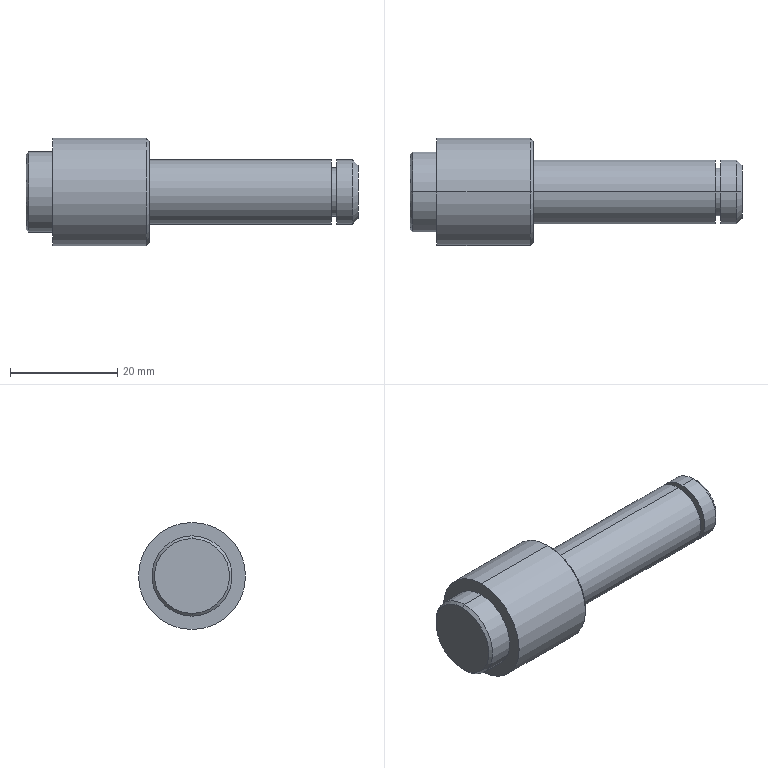Part | STEP file | 1 solid | 22 faces | box 62 x 20 x 20 mm | volume 10868 mm3 | cylinder 10 | cone 6 | plane 6 | commonest cylinder face diameters 12 x4 9 x2 15 x2 20 x2
STEP:
#1=CARTESIAN_POINT('',(0.,0.,0.));
#2=DIRECTION('',(0.,0.,1.));
#3=DIRECTION('',(1.,0.,0.));
#4=AXIS2_PLACEMENT_3D('',#1,#2,#3);
#5=CARTESIAN_POINT('',(23.,0.,-6.));
#6=VERTEX_POINT('',#5);
#7=CARTESIAN_POINT('',(23.,0.,6.));
#8=VERTEX_POINT('',#7);
#9=CARTESIAN_POINT('',(23.,0.,0.));
#10=DIRECTION('',(1.,0.,0.));
#11=DIRECTION('',(0.,0.,-1.));
#12=AXIS2_PLACEMENT_3D('',#9,#10,#11);
#13=CIRCLE('',#12,6.);
#14=CARTESIAN_POINT('',(40.,0.,0.));
#15=DIRECTION('',(1.,0.,0.));
#16=DIRECTION('',(0.,0.,-1.));
#17=AXIS2_PLACEMENT_3D('',#14,#15,#16);
#18=CYLINDRICAL_SURFACE('',#17,6.);
#19=CARTESIAN_POINT('',(0.,-17.));
#20=DIRECTION('',(1.,0.));
#21=VECTOR('',#20,1.);
#22=LINE('',#19,#21);
#23=(GEOMETRIC_REPRESENTATION_CONTEXT(2)PARAMETRIC_REPRESENTATION_CONTEXT()REPRESENTATION_CONTEXT('',''));
#24=DEFINITIONAL_REPRESENTATION('',(#22),#23);
#25=PCURVE('',#18,#24);
#26=CARTESIAN_POINT('',(23.,8.,0.));
#27=DIRECTION('',(1.,0.,0.));
#28=DIRECTION('',(0.,0.,-1.));
#29=AXIS2_PLACEMENT_3D('',#26,#27,#28);
#30=PLANE('',#29);
#31=CARTESIAN_POINT('',(0.,-8.));
#32=DIRECTION('',(1.,0.));
#33=AXIS2_PLACEMENT_2D('',#31,#32);
#34=CIRCLE('',#33,6.);
#35=(GEOMETRIC_REPRESENTATION_CONTEXT(2)PARAMETRIC_REPRESENTATION_CONTEXT()REPRESENTATION_CONTEXT('',''));
#36=DEFINITIONAL_REPRESENTATION('',(#34),#35);
#37=PCURVE('',#30,#36);
#38=SURFACE_CURVE('',#13,(#25,#37),.PCURVE_S1.);
#39=EDGE_CURVE('',#6,#8,#38,.T.);
#40=ORIENTED_EDGE('',*,*,#39,.T.);
#41=CARTESIAN_POINT('',(57.,0.,6.));
#42=VERTEX_POINT('',#41);
#43=CARTESIAN_POINT('',(40.,0.,6.));
#44=DIRECTION('',(1.,0.,0.));
#45=VECTOR('',#44,1.);
#46=LINE('',#43,#45);
#47=CARTESIAN_POINT('',(3.142,0.));
#48=DIRECTION('',(0.,1.));
#49=VECTOR('',#48,1.);
#50=LINE('',#47,#49);
#51=(GEOMETRIC_REPRESENTATION_CONTEXT(2)PARAMETRIC_REPRESENTATION_CONTEXT()REPRESENTATION_CONTEXT('',''));
#52=DEFINITIONAL_REPRESENTATION('',(#50),#51);
#53=PCURVE('',#18,#52);
#54=CARTESIAN_POINT('',(40.,0.,0.));
#55=DIRECTION('',(1.,0.,0.));
#56=DIRECTION('',(0.,0.,-1.));
#57=AXIS2_PLACEMENT_3D('',#54,#55,#56);
#58=CYLINDRICAL_SURFACE('',#57,6.);
#59=CARTESIAN_POINT('',(3.142,0.));
#60=DIRECTION('',(0.,1.));
#61=VECTOR('',#60,1.);
#62=LINE('',#59,#61);
#63=(GEOMETRIC_REPRESENTATION_CONTEXT(2)PARAMETRIC_REPRESENTATION_CONTEXT()REPRESENTATION_CONTEXT('',''));
#64=DEFINITIONAL_REPRESENTATION('',(#62),#63);
#65=PCURVE('',#58,#64);
#66=SURFACE_CURVE('',#46,(#53,#65),.PCURVE_S1.);
#67=EDGE_CURVE('',#8,#42,#66,.T.);
#68=ORIENTED_EDGE('',*,*,#67,.T.);
#69=CARTESIAN_POINT('',(57.,0.,-6.));
#70=VERTEX_POINT('',#69);
#71=CARTESIAN_POINT('',(57.,0.,0.));
#72=DIRECTION('',(-1.,0.,0.));
#73=DIRECTION('',(0.,0.,-1.));
#74=AXIS2_PLACEMENT_3D('',#71,#72,#73);
#75=CIRCLE('',#74,6.);
#76=CARTESIAN_POINT('',(6.283,17.));
#77=DIRECTION('',(-1.,0.));
#78=VECTOR('',#77,1.);
#79=LINE('',#76,#78);
#80=(GEOMETRIC_REPRESENTATION_CONTEXT(2)PARAMETRIC_REPRESENTATION_CONTEXT()REPRESENTATION_CONTEXT('',''));
#81=DEFINITIONAL_REPRESENTATION('',(#79),#80);
#82=PCURVE('',#18,#81);
#83=CARTESIAN_POINT('',(57.,5.25,0.));
#84=DIRECTION('',(1.,0.,0.));
#85=DIRECTION('',(0.,0.,-1.));
#86=AXIS2_PLACEMENT_3D('',#83,#84,#85);
#87=PLANE('',#86);
#88=CARTESIAN_POINT('',(6.,-5.25));
#89=CARTESIAN_POINT('',(6.,-15.642));
#90=CARTESIAN_POINT('',(-3.,-10.446));
#91=CARTESIAN_POINT('',(-12.,-5.25));
#92=CARTESIAN_POINT('',(-3.,-0.05385));
#93=CARTESIAN_POINT('',(6.,5.142));
#94=CARTESIAN_POINT('',(6.,-5.25));
#95=(BOUNDED_CURVE()B_SPLINE_CURVE(2,(#88,#89,#90,#91,#92,#93,#94),.UNSPECIFIED.,.T.,.F.)B_SPLINE_CURVE_WITH_KNOTS((1,2,2,2,2,1),(-2.094,0.,2.094,4.189,6.283,8.378),.UNSPECIFIED.)CURVE()GEOMETRIC_REPRESENTATION_ITEM()RATIONAL_B_SPLINE_CURVE((1.,0.5,1.,0.5,1.,0.5,1.))REPRESENTATION_ITEM(''));
#96=(GEOMETRIC_REPRESENTATION_CONTEXT(2)PARAMETRIC_REPRESENTATION_CONTEXT()REPRESENTATION_CONTEXT('',''));
#97=DEFINITIONAL_REPRESENTATION('',(#95),#96);
#98=PCURVE('',#87,#97);
#99=SURFACE_CURVE('',#75,(#82,#98),.PCURVE_S1.);
#100=EDGE_CURVE('',#42,#70,#99,.T.);
#101=ORIENTED_EDGE('',*,*,#100,.T.);
#102=CARTESIAN_POINT('',(40.,0.,-6.));
#103=DIRECTION('',(1.,0.,0.));
#104=VECTOR('',#103,1.);
#105=LINE('',#102,#104);
#106=CARTESIAN_POINT('',(0.,0.));
#107=DIRECTION('',(0.,1.));
#108=VECTOR('',#107,1.);
#109=LINE('',#106,#108);
#110=(GEOMETRIC_REPRESENTATION_CONTEXT(2)PARAMETRIC_REPRESENTATION_CONTEXT()REPRESENTATION_CONTEXT('',''));
#111=DEFINITIONAL_REPRESENTATION('',(#109),#110);
#112=PCURVE('',#18,#111);
#113=CARTESIAN_POINT('',(6.283,0.));
#114=DIRECTION('',(0.,1.));
#115=VECTOR('',#114,1.);
#116=LINE('',#113,#115);
#117=(GEOMETRIC_REPRESENTATION_CONTEXT(2)PARAMETRIC_REPRESENTATION_CONTEXT()REPRESENTATION_CONTEXT('',''));
#118=DEFINITIONAL_REPRESENTATION('',(#116),#117);
#119=PCURVE('',#58,#118);
#120=SURFACE_CURVE('',#105,(#112,#119),.PCURVE_S1.);
#121=EDGE_CURVE('',#6,#70,#120,.T.);
#122=ORIENTED_EDGE('',*,*,#121,.F.);
#123=EDGE_LOOP('',(#40,#68,#101,#122));
#124=FACE_BOUND('',#123,.T.);
#125=ADVANCED_FACE('',(#124),#18,.T.);
#126=CARTESIAN_POINT('',(23.,0.,-9.5));
#127=VERTEX_POINT('',#126);
#128=CARTESIAN_POINT('',(23.,0.,9.5));
#129=VERTEX_POINT('',#128);
#130=CARTESIAN_POINT('',(23.,0.,0.));
#131=DIRECTION('',(1.,0.,0.));
#132=DIRECTION('',(0.,0.,1.));
#133=AXIS2_PLACEMENT_3D('',#130,#131,#132);
#134=CIRCLE('',#133,9.5);
#135=CARTESIAN_POINT('',(22.5,0.,0.));
#136=DIRECTION('',(-1.,0.,0.));
#137=DIRECTION('',(0.,0.,1.));
#138=AXIS2_PLACEMENT_3D('',#135,#136,#137);
#139=CONICAL_SURFACE('',#138,10.,0.7854);
#140=CARTESIAN_POINT('',(6.283,-0.5));
#141=DIRECTION('',(-1.,0.));
#142=VECTOR('',#141,1.);
#143=LINE('',#140,#142);
#144=(GEOMETRIC_REPRESENTATION_CONTEXT(2)PARAMETRIC_REPRESENTATION_CONTEXT()REPRESENTATION_CONTEXT('',''));
#145=DEFINITIONAL_REPRESENTATION('',(#143),#144);
#146=PCURVE('',#139,#145);
#147=CARTESIAN_POINT('',(0.,-8.));
#148=DIRECTION('',(-1.,0.));
#149=AXIS2_PLACEMENT_2D('',#147,#148);
#150=CIRCLE('',#149,9.5);
#151=(GEOMETRIC_REPRESENTATION_CONTEXT(2)PARAMETRIC_REPRESENTATION_CONTEXT()REPRESENTATION_CONTEXT('',''));
#152=DEFINITIONAL_REPRESENTATION('',(#150),#151);
#153=PCURVE('',#30,#152);
#154=SURFACE_CURVE('',#134,(#146,#153),.PCURVE_S1.);
#155=EDGE_CURVE('',#127,#129,#154,.T.);
#156=ORIENTED_EDGE('',*,*,#155,.F.);
#157=CARTESIAN_POINT('',(22.5,0.,-10.));
#158=VERTEX_POINT('',#157);
#159=CARTESIAN_POINT('',(22.5,0.,-10.));
#160=DIRECTION('',(-0.7071,0.,-0.7071));
#161=VECTOR('',#160,1.);
#162=LINE('',#159,#161);
#163=CARTESIAN_POINT('',(3.142,0.));
#164=DIRECTION('',(0.,1.));
#165=VECTOR('',#164,1.);
#166=LINE('',#163,#165);
#167=(GEOMETRIC_REPRESENTATION_CONTEXT(2)PARAMETRIC_REPRESENTATION_CONTEXT()REPRESENTATION_CONTEXT('',''));
#168=DEFINITIONAL_REPRESENTATION('',(#166),#167);
#169=PCURVE('',#139,#168);
#170=CARTESIAN_POINT('',(22.5,0.,0.));
#171=DIRECTION('',(-1.,0.,0.));
#172=DIRECTION('',(0.,0.,1.));
#173=AXIS2_PLACEMENT_3D('',#170,#171,#172);
#174=CONICAL_SURFACE('',#173,10.,0.7854);
#175=CARTESIAN_POINT('',(3.142,0.));
#176=DIRECTION('',(0.,1.));
#177=VECTOR('',#176,1.);
#178=LINE('',#175,#177);
#179=(GEOMETRIC_REPRESENTATION_CONTEXT(2)PARAMETRIC_REPRESENTATION_CONTEXT()REPRESENTATION_CONTEXT('',''));
#180=DEFINITIONAL_REPRESENTATION('',(#178),#179);
#181=PCURVE('',#174,#180);
#182=SURFACE_CURVE('',#162,(#169,#181),.PCURVE_S1.);
#183=EDGE_CURVE('',#127,#158,#182,.T.);
#184=ORIENTED_EDGE('',*,*,#183,.T.);
#185=CARTESIAN_POINT('',(22.5,0.,10.));
#186=VERTEX_POINT('',#185);
#187=CARTESIAN_POINT('',(22.5,0.,0.));
#188=DIRECTION('',(1.,0.,0.));
#189=DIRECTION('',(0.,-1.,0.));
#190=AXIS2_PLACEMENT_3D('',#187,#188,#189);
#191=CIRCLE('',#190,10.);
#192=CARTESIAN_POINT('',(4.712,0.));
#193=DIRECTION('',(-1.,0.));
#194=VECTOR('',#193,1.);
#195=LINE('',#192,#194);
#196=(GEOMETRIC_REPRESENTATION_CONTEXT(2)PARAMETRIC_REPRESENTATION_CONTEXT()REPRESENTATION_CONTEXT('',''));
#197=DEFINITIONAL_REPRESENTATION('',(#195),#196);
#198=PCURVE('',#139,#197);
#199=CARTESIAN_POINT('',(14.,0.,0.));
#200=DIRECTION('',(1.,0.,0.));
#201=DIRECTION('',(0.,0.,-1.));
#202=AXIS2_PLACEMENT_3D('',#199,#200,#201);
#203=CYLINDRICAL_SURFACE('',#202,10.);
#204=CARTESIAN_POINT('',(-1.571,8.5));
#205=DIRECTION('',(1.,0.));
#206=VECTOR('',#205,1.);
#207=LINE('',#204,#206);
#208=(GEOMETRIC_REPRESENTATION_CONTEXT(2)PARAMETRIC_REPRESENTATION_CONTEXT()REPRESENTATION_CONTEXT('',''));
#209=DEFINITIONAL_REPRESENTATION('',(#207),#208);
#210=PCURVE('',#203,#209);
#211=SURFACE_CURVE('',#191,(#198,#210),.PCURVE_S1.);
#212=EDGE_CURVE('',#158,#186,#211,.T.);
#213=ORIENTED_EDGE('',*,*,#212,.T.);
#214=CARTESIAN_POINT('',(22.5,0.,10.));
#215=DIRECTION('',(-0.7071,0.,0.7071));
#216=VECTOR('',#215,1.);
#217=LINE('',#214,#216);
#218=CARTESIAN_POINT('',(0.,0.));
#219=DIRECTION('',(0.,1.));
#220=VECTOR('',#219,1.);
#221=LINE('',#218,#220);
#222=(GEOMETRIC_REPRESENTATION_CONTEXT(2)PARAMETRIC_REPRESENTATION_CONTEXT()REPRESENTATION_CONTEXT('',''));
#223=DEFINITIONAL_REPRESENTATION('',(#221),#222);
#224=PCURVE('',#139,#223);
#225=CARTESIAN_POINT('',(6.283,0.));
#226=DIRECTION('',(0.,1.));
#227=VECTOR('',#226,1.);
#228=LINE('',#225,#227);
#229=(GEOMETRIC_REPRESENTATION_CONTEXT(2)PARAMETRIC_REPRESENTATION_CONTEXT()REPRESENTATION_CONTEXT('',''));
#230=DEFINITIONAL_REPRESENTATION('',(#228),#229);
#231=PCURVE('',#174,#230);
#232=SURFACE_CURVE('',#217,(#224,#231),.PCURVE_S1.);
#233=EDGE_CURVE('',#129,#186,#232,.T.);
#234=ORIENTED_EDGE('',*,*,#233,.F.);
#235=EDGE_LOOP('',(#156,#184,#213,#234));
#236=FACE_BOUND('',#235,.T.);
#237=ADVANCED_FACE('',(#236),#139,.T.);
#238=CARTESIAN_POINT('',(57.,0.,4.5));
#239=VERTEX_POINT('',#238);
#240=CARTESIAN_POINT('',(57.,0.,-4.5));
#241=VERTEX_POINT('',#240);
#242=CARTESIAN_POINT('',(57.,0.,0.));
#243=DIRECTION('',(-1.,0.,0.));
#244=DIRECTION('',(0.,0.,-1.));
#245=AXIS2_PLACEMENT_3D('',#242,#243,#244);
#246=CIRCLE('',#245,4.5);
#247=CARTESIAN_POINT('',(57.5,0.,0.));
#248=DIRECTION('',(1.,0.,0.));
#249=DIRECTION('',(0.,0.,-1.));
#250=AXIS2_PLACEMENT_3D('',#247,#248,#249);
#251=CYLINDRICAL_SURFACE('',#250,4.5);
#252=CARTESIAN_POINT('',(6.283,-0.5));
#253=DIRECTION('',(-1.,0.));
#254=VECTOR('',#253,1.);
#255=LINE('',#252,#254);
#256=(GEOMETRIC_REPRESENTATION_CONTEXT(2)PARAMETRIC_REPRESENTATION_CONTEXT()REPRESENTATION_CONTEXT('',''));
#257=DEFINITIONAL_REPRESENTATION('',(#255),#256);
#258=PCURVE('',#251,#257);
#259=CARTESIAN_POINT('',(4.5,-5.25));
#260=CARTESIAN_POINT('',(4.5,-13.044));
#261=CARTESIAN_POINT('',(-2.25,-9.147));
#262=CARTESIAN_POINT('',(-9.,-5.25));
#263=CARTESIAN_POINT('',(-2.25,-1.353));
#264=CARTESIAN_POINT('',(4.5,2.544));
#265=CARTESIAN_POINT('',(4.5,-5.25));
#266=(BOUNDED_CURVE()B_SPLINE_CURVE(2,(#259,#260,#261,#262,#263,#264,#265),.UNSPECIFIED.,.T.,.F.)B_SPLINE_CURVE_WITH_KNOTS((1,2,2,2,2,1),(-2.094,0.,2.094,4.189,6.283,8.378),.UNSPECIFIED.)CURVE()GEOMETRIC_REPRESENTATION_ITEM()RATIONAL_B_SPLINE_CURVE((1.,0.5,1.,0.5,1.,0.5,1.))REPRESENTATION_ITEM(''));
#267=(GEOMETRIC_REPRESENTATION_CONTEXT(2)PARAMETRIC_REPRESENTATION_CONTEXT()REPRESENTATION_CONTEXT('',''));
#268=DEFINITIONAL_REPRESENTATION('',(#266),#267);
#269=PCURVE('',#87,#268);
#270=SURFACE_CURVE('',#246,(#258,#269),.PCURVE_S1.);
#271=EDGE_CURVE('',#239,#241,#270,.T.);
#272=ORIENTED_EDGE('',*,*,#271,.F.);
#273=CARTESIAN_POINT('',(58.,0.,4.5));
#274=VERTEX_POINT('',#273);
#275=CARTESIAN_POINT('',(57.5,0.,4.5));
#276=DIRECTION('',(1.,0.,0.));
#277=VECTOR('',#276,1.);
#278=LINE('',#275,#277);
#279=CARTESIAN_POINT('',(3.142,0.));
#280=DIRECTION('',(0.,1.));
#281=VECTOR('',#280,1.);
#282=LINE('',#279,#281);
#283=(GEOMETRIC_REPRESENTATION_CONTEXT(2)PARAMETRIC_REPRESENTATION_CONTEXT()REPRESENTATION_CONTEXT('',''));
#284=DEFINITIONAL_REPRESENTATION('',(#282),#283);
#285=PCURVE('',#251,#284);
#286=CARTESIAN_POINT('',(57.5,0.,0.));
#287=DIRECTION('',(1.,0.,0.));
#288=DIRECTION('',(0.,0.,-1.));
#289=AXIS2_PLACEMENT_3D('',#286,#287,#288);
#290=CYLINDRICAL_SURFACE('',#289,4.5);
#291=CARTESIAN_POINT('',(3.142,0.));
#292=DIRECTION('',(0.,1.));
#293=VECTOR('',#292,1.);
#294=LINE('',#291,#293);
#295=(GEOMETRIC_REPRESENTATION_CONTEXT(2)PARAMETRIC_REPRESENTATION_CONTEXT()REPRESENTATION_CONTEXT('',''));
#296=DEFINITIONAL_REPRESENTATION('',(#294),#295);
#297=PCURVE('',#290,#296);
#298=SURFACE_CURVE('',#278,(#285,#297),.PCURVE_S1.);
#299=EDGE_CURVE('',#239,#274,#298,.T.);
#300=ORIENTED_EDGE('',*,*,#299,.T.);
#301=CARTESIAN_POINT('',(58.,0.,-4.5));
#302=VERTEX_POINT('',#301);
#303=CARTESIAN_POINT('',(58.,0.,0.));
#304=DIRECTION('',(-1.,0.,0.));
#305=DIRECTION('',(0.,0.,-1.));
#306=AXIS2_PLACEMENT_3D('',#303,#304,#305);
#307=CIRCLE('',#306,4.5);
#308=CARTESIAN_POINT('',(6.283,0.5));
#309=DIRECTION('',(-1.,0.));
#310=VECTOR('',#309,1.);
#311=LINE('',#308,#310);
#312=(GEOMETRIC_REPRESENTATION_CONTEXT(2)PARAMETRIC_REPRESENTATION_CONTEXT()REPRESENTATION_CONTEXT('',''));
#313=DEFINITIONAL_REPRESENTATION('',(#311),#312);
#314=PCURVE('',#251,#313);
#315=CARTESIAN_POINT('',(58.,5.25,0.));
#316=DIRECTION('',(-1.,0.,0.));
#317=DIRECTION('',(0.,0.,1.));
#318=AXIS2_PLACEMENT_3D('',#315,#316,#317);
#319=PLANE('',#318);
#320=CARTESIAN_POINT('',(0.,-5.25));
#321=DIRECTION('',(-1.,0.));
#322=AXIS2_PLACEMENT_2D('',#320,#321);
#323=CIRCLE('',#322,4.5);
#324=(GEOMETRIC_REPRESENTATION_CONTEXT(2)PARAMETRIC_REPRESENTATION_CONTEXT()REPRESENTATION_CONTEXT('',''));
#325=DEFINITIONAL_REPRESENTATION('',(#323),#324);
#326=PCURVE('',#319,#325);
#327=SURFACE_CURVE('',#307,(#314,#326),.PCURVE_S1.);
#328=EDGE_CURVE('',#274,#302,#327,.T.);
#329=ORIENTED_EDGE('',*,*,#328,.T.);
#330=CARTESIAN_POINT('',(57.5,0.,-4.5));
#331=DIRECTION('',(1.,0.,0.));
#332=VECTOR('',#331,1.);
#333=LINE('',#330,#332);
#334=CARTESIAN_POINT('',(0.,0.));
#335=DIRECTION('',(0.,1.));
#336=VECTOR('',#335,1.);
#337=LINE('',#334,#336);
#338=(GEOMETRIC_REPRESENTATION_CONTEXT(2)PARAMETRIC_REPRESENTATION_CONTEXT()REPRESENTATION_CONTEXT('',''));
#339=DEFINITIONAL_REPRESENTATION('',(#337),#338);
#340=PCURVE('',#251,#339);
#341=CARTESIAN_POINT('',(6.283,0.));
#342=DIRECTION('',(0.,1.));
#343=VECTOR('',#342,1.);
#344=LINE('',#341,#343);
#345=(GEOMETRIC_REPRESENTATION_CONTEXT(2)PARAMETRIC_REPRESENTATION_CONTEXT()REPRESENTATION_CONTEXT('',''));
#346=DEFINITIONAL_REPRESENTATION('',(#344),#345);
#347=PCURVE('',#290,#346);
#348=SURFACE_CURVE('',#333,(#340,#347),.PCURVE_S1.);
#349=EDGE_CURVE('',#241,#302,#348,.T.);
#350=ORIENTED_EDGE('',*,*,#349,.F.);
#351=EDGE_LOOP('',(#272,#300,#329,#350));
#352=FACE_BOUND('',#351,.T.);
#353=ADVANCED_FACE('',(#352),#251,.T.);
#354=CARTESIAN_POINT('',(5.,0.,-10.));
#355=VERTEX_POINT('',#354);
#356=CARTESIAN_POINT('',(5.,0.,10.));
#357=VERTEX_POINT('',#356);
#358=CARTESIAN_POINT('',(5.,0.,0.));
#359=DIRECTION('',(1.,0.,0.));
#360=DIRECTION('',(0.,0.,-1.));
#361=AXIS2_PLACEMENT_3D('',#358,#359,#360);
#362=CIRCLE('',#361,10.);
#363=CARTESIAN_POINT('',(0.,-9.));
#364=DIRECTION('',(1.,0.));
#365=VECTOR('',#364,1.);
#366=LINE('',#363,#365);
#367=(GEOMETRIC_REPRESENTATION_CONTEXT(2)PARAMETRIC_REPRESENTATION_CONTEXT()REPRESENTATION_CONTEXT('',''));
#368=DEFINITIONAL_REPRESENTATION('',(#366),#367);
#369=PCURVE('',#203,#368);
#370=CARTESIAN_POINT('',(5.,8.75,0.));
#371=DIRECTION('',(-1.,0.,0.));
#372=DIRECTION('',(0.,0.,1.));
#373=AXIS2_PLACEMENT_3D('',#370,#371,#372);
#374=PLANE('',#373);
#375=CARTESIAN_POINT('',(-10.,-8.75));
#376=CARTESIAN_POINT('',(-10.,8.571));
#377=CARTESIAN_POINT('',(5.,-0.08975));
#378=CARTESIAN_POINT('',(20.,-8.75));
#379=CARTESIAN_POINT('',(5.,-17.41));
#380=CARTESIAN_POINT('',(-10.,-26.071));
#381=CARTESIAN_POINT('',(-10.,-8.75));
#382=(BOUNDED_CURVE()B_SPLINE_CURVE(2,(#375,#376,#377,#378,#379,#380,#381),.UNSPECIFIED.,.T.,.F.)B_SPLINE_CURVE_WITH_KNOTS((1,2,2,2,2,1),(-2.094,0.,2.094,4.189,6.283,8.378),.UNSPECIFIED.)CURVE()GEOMETRIC_REPRESENTATION_ITEM()RATIONAL_B_SPLINE_CURVE((1.,0.5,1.,0.5,1.,0.5,1.))REPRESENTATION_ITEM(''));
#383=(GEOMETRIC_REPRESENTATION_CONTEXT(2)PARAMETRIC_REPRESENTATION_CONTEXT()REPRESENTATION_CONTEXT('',''));
#384=DEFINITIONAL_REPRESENTATION('',(#382),#383);
#385=PCURVE('',#374,#384);
#386=SURFACE_CURVE('',#362,(#369,#385),.PCURVE_S1.);
#387=EDGE_CURVE('',#355,#357,#386,.T.);
#388=ORIENTED_EDGE('',*,*,#387,.T.);
#389=CARTESIAN_POINT('',(14.,0.,10.));
#390=DIRECTION('',(1.,0.,0.));
#391=VECTOR('',#390,1.);
#392=LINE('',#389,#391);
#393=CARTESIAN_POINT('',(3.142,0.));
#394=DIRECTION('',(0.,1.));
#395=VECTOR('',#394,1.);
#396=LINE('',#393,#395);
#397=(GEOMETRIC_REPRESENTATION_CONTEXT(2)PARAMETRIC_REPRESENTATION_CONTEXT()REPRESENTATION_CONTEXT('',''));
#398=DEFINITIONAL_REPRESENTATION('',(#396),#397);
#399=PCURVE('',#203,#398);
#400=CARTESIAN_POINT('',(14.,0.,0.));
#401=DIRECTION('',(1.,0.,0.));
#402=DIRECTION('',(0.,0.,-1.));
#403=AXIS2_PLACEMENT_3D('',#400,#401,#402);
#404=CYLINDRICAL_SURFACE('',#403,10.);
#405=CARTESIAN_POINT('',(3.142,0.));
#406=DIRECTION('',(0.,1.));
#407=VECTOR('',#406,1.);
#408=LINE('',#405,#407);
#409=(GEOMETRIC_REPRESENTATION_CONTEXT(2)PARAMETRIC_REPRESENTATION_CONTEXT()REPRESENTATION_CONTEXT('',''));
#410=DEFINITIONAL_REPRESENTATION('',(#408),#409);
#411=PCURVE('',#404,#410);
#412=SURFACE_CURVE('',#392,(#399,#411),.PCURVE_S1.);
#413=EDGE_CURVE('',#357,#186,#412,.T.);
#414=ORIENTED_EDGE('',*,*,#413,.T.);
#415=ORIENTED_EDGE('',*,*,#212,.F.);
#416=CARTESIAN_POINT('',(14.,0.,-10.));
#417=DIRECTION('',(1.,0.,0.));
#418=VECTOR('',#417,1.);
#419=LINE('',#416,#418);
#420=CARTESIAN_POINT('',(0.,0.));
#421=DIRECTION('',(0.,1.));
#422=VECTOR('',#421,1.);
#423=LINE('',#420,#422);
#424=(GEOMETRIC_REPRESENTATION_CONTEXT(2)PARAMETRIC_REPRESENTATION_CONTEXT()REPRESENTATION_CONTEXT('',''));
#425=DEFINITIONAL_REPRESENTATION('',(#423),#424);
#426=PCURVE('',#203,#425);
#427=CARTESIAN_POINT('',(6.283,0.));
#428=DIRECTION('',(0.,1.));
#429=VECTOR('',#428,1.);
#430=LINE('',#427,#429);
#431=(GEOMETRIC_REPRESENTATION_CONTEXT(2)PARAMETRIC_REPRESENTATION_CONTEXT()REPRESENTATION_CONTEXT('',''));
#432=DEFINITIONAL_REPRESENTATION('',(#430),#431);
#433=PCURVE('',#404,#432);
#434=SURFACE_CURVE('',#419,(#426,#433),.PCURVE_S1.);
#435=EDGE_CURVE('',#355,#158,#434,.T.);
#436=ORIENTED_EDGE('',*,*,#435,.F.);
#437=EDGE_LOOP('',(#388,#414,#415,#436));
#438=FACE_BOUND('',#437,.T.);
#439=ADVANCED_FACE('',(#438),#203,.T.);
#440=CARTESIAN_POINT('',(58.,0.,6.));
#441=VERTEX_POINT('',#440);
#442=CARTESIAN_POINT('',(58.,0.,-6.));
#443=VERTEX_POINT('',#442);
#444=CARTESIAN_POINT('',(58.,0.,0.));
#445=DIRECTION('',(-1.,0.,0.));
#446=DIRECTION('',(0.,0.,-1.));
#447=AXIS2_PLACEMENT_3D('',#444,#445,#446);
#448=CIRCLE('',#447,6.);
#449=CARTESIAN_POINT('',(59.5,0.,0.));
#450=DIRECTION('',(1.,0.,0.));
#451=DIRECTION('',(0.,0.,-1.));
#452=AXIS2_PLACEMENT_3D('',#449,#450,#451);
#453=CYLINDRICAL_SURFACE('',#452,6.);
#454=CARTESIAN_POINT('',(6.283,-1.5));
#455=DIRECTION('',(-1.,0.));
#456=VECTOR('',#455,1.);
#457=LINE('',#454,#456);
#458=(GEOMETRIC_REPRESENTATION_CONTEXT(2)PARAMETRIC_REPRESENTATION_CONTEXT()REPRESENTATION_CONTEXT('',''));
#459=DEFINITIONAL_REPRESENTATION('',(#457),#458);
#460=PCURVE('',#453,#459);
#461=CARTESIAN_POINT('',(0.,-5.25));
#462=DIRECTION('',(-1.,0.));
#463=AXIS2_PLACEMENT_2D('',#461,#462);
#464=CIRCLE('',#463,6.);
#465=(GEOMETRIC_REPRESENTATION_CONTEXT(2)PARAMETRIC_REPRESENTATION_CONTEXT()REPRESENTATION_CONTEXT('',''));
#466=DEFINITIONAL_REPRESENTATION('',(#464),#465);
#467=PCURVE('',#319,#466);
#468=SURFACE_CURVE('',#448,(#460,#467),.PCURVE_S1.);
#469=EDGE_CURVE('',#441,#443,#468,.T.);
#470=ORIENTED_EDGE('',*,*,#469,.F.);
#471=CARTESIAN_POINT('',(61.,0.,6.));
#472=VERTEX_POINT('',#471);
#473=CARTESIAN_POINT('',(59.5,0.,6.));
#474=DIRECTION('',(1.,0.,0.));
#475=VECTOR('',#474,1.);
#476=LINE('',#473,#475);
#477=CARTESIAN_POINT('',(3.142,0.));
#478=DIRECTION('',(0.,1.));
#479=VECTOR('',#478,1.);
#480=LINE('',#477,#479);
#481=(GEOMETRIC_REPRESENTATION_CONTEXT(2)PARAMETRIC_REPRESENTATION_CONTEXT()REPRESENTATION_CONTEXT('',''));
#482=DEFINITIONAL_REPRESENTATION('',(#480),#481);
#483=PCURVE('',#453,#482);
#484=CARTESIAN_POINT('',(59.5,0.,0.));
#485=DIRECTION('',(1.,0.,0.));
#486=DIRECTION('',(0.,0.,-1.));
#487=AXIS2_PLACEMENT_3D('',#484,#485,#486);
#488=CYLINDRICAL_SURFACE('',#487,6.);
#489=CARTESIAN_POINT('',(3.142,0.));
#490=DIRECTION('',(0.,1.));
#491=VECTOR('',#490,1.);
#492=LINE('',#489,#491);
#493=(GEOMETRIC_REPRESENTATION_CONTEXT(2)PARAMETRIC_REPRESENTATION_CONTEXT()REPRESENTATION_CONTEXT('',''));
#494=DEFINITIONAL_REPRESENTATION('',(#492),#493);
#495=PCURVE('',#488,#494);
#496=SURFACE_CURVE('',#476,(#483,#495),.PCURVE_S1.);
#497=EDGE_CURVE('',#441,#472,#496,.T.);
#498=ORIENTED_EDGE('',*,*,#497,.T.);
#499=CARTESIAN_POINT('',(61.,0.,-6.));
#500=VERTEX_POINT('',#499);
#501=CARTESIAN_POINT('',(61.,0.,0.));
#502=DIRECTION('',(-1.,0.,0.));
#503=DIRECTION('',(0.,0.,-1.));
#504=AXIS2_PLACEMENT_3D('',#501,#502,#503);
#505=CIRCLE('',#504,6.);
#506=CARTESIAN_POINT('',(6.283,1.5));
#507=DIRECTION('',(-1.,0.));
#508=VECTOR('',#507,1.);
#509=LINE('',#506,#508);
#510=(GEOMETRIC_REPRESENTATION_CONTEXT(2)PARAMETRIC_REPRESENTATION_CONTEXT()REPRESENTATION_CONTEXT('',''));
#511=DEFINITIONAL_REPRESENTATION('',(#509),#510);
#512=PCURVE('',#453,#511);
#513=CARTESIAN_POINT('',(61.,0.,0.));
#514=DIRECTION('',(-1.,0.,0.));
#515=DIRECTION('',(0.,0.,1.));
#516=AXIS2_PLACEMENT_3D('',#513,#514,#515);
#517=CONICAL_SURFACE('',#516,6.,0.7854);
#518=CARTESIAN_POINT('',(-3.142,0.));
#519=DIRECTION('',(1.,0.));
#520=VECTOR('',#519,1.);
#521=LINE('',#518,#520);
#522=(GEOMETRIC_REPRESENTATION_CONTEXT(2)PARAMETRIC_REPRESENTATION_CONTEXT()REPRESENTATION_CONTEXT('',''));
#523=DEFINITIONAL_REPRESENTATION('',(#521),#522);
#524=PCURVE('',#517,#523);
#525=SURFACE_CURVE('',#505,(#512,#524),.PCURVE_S1.);
#526=EDGE_CURVE('',#472,#500,#525,.T.);
#527=ORIENTED_EDGE('',*,*,#526,.T.);
#528=CARTESIAN_POINT('',(59.5,0.,-6.));
#529=DIRECTION('',(1.,0.,0.));
#530=VECTOR('',#529,1.);
#531=LINE('',#528,#530);
#532=CARTESIAN_POINT('',(0.,0.));
#533=DIRECTION('',(0.,1.));
#534=VECTOR('',#533,1.);
#535=LINE('',#532,#534);
#536=(GEOMETRIC_REPRESENTATION_CONTEXT(2)PARAMETRIC_REPRESENTATION_CONTEXT()REPRESENTATION_CONTEXT('',''));
#537=DEFINITIONAL_REPRESENTATION('',(#535),#536);
#538=PCURVE('',#453,#537);
#539=CARTESIAN_POINT('',(6.283,0.));
#540=DIRECTION('',(0.,1.));
#541=VECTOR('',#540,1.);
#542=LINE('',#539,#541);
#543=(GEOMETRIC_REPRESENTATION_CONTEXT(2)PARAMETRIC_REPRESENTATION_CONTEXT()REPRESENTATION_CONTEXT('',''));
#544=DEFINITIONAL_REPRESENTATION('',(#542),#543);
#545=PCURVE('',#488,#544);
#546=SURFACE_CURVE('',#531,(#538,#545),.PCURVE_S1.);
#547=EDGE_CURVE('',#443,#500,#546,.T.);
#548=ORIENTED_EDGE('',*,*,#547,.F.);
#549=EDGE_LOOP('',(#470,#498,#527,#548));
#550=FACE_BOUND('',#549,.T.);
#551=ADVANCED_FACE('',(#550),#453,.T.);
#552=CARTESIAN_POINT('',(0.5,0.,-7.5));
#553=VERTEX_POINT('',#552);
#554=CARTESIAN_POINT('',(0.5,0.,7.5));
#555=VERTEX_POINT('',#554);
#556=CARTESIAN_POINT('',(0.5,0.,0.));
#557=DIRECTION('',(1.,0.,0.));
#558=DIRECTION('',(0.,0.,-1.));
#559=AXIS2_PLACEMENT_3D('',#556,#557,#558);
#560=CIRCLE('',#559,7.5);
#561=CARTESIAN_POINT('',(2.5,0.,0.));
#562=DIRECTION('',(1.,0.,0.));
#563=DIRECTION('',(0.,0.,-1.));
#564=AXIS2_PLACEMENT_3D('',#561,#562,#563);
#565=CYLINDRICAL_SURFACE('',#564,7.5);
#566=CARTESIAN_POINT('',(0.,-2.));
#567=DIRECTION('',(1.,0.));
#568=VECTOR('',#567,1.);
#569=LINE('',#566,#568);
#570=(GEOMETRIC_REPRESENTATION_CONTEXT(2)PARAMETRIC_REPRESENTATION_CONTEXT()REPRESENTATION_CONTEXT('',''));
#571=DEFINITIONAL_REPRESENTATION('',(#569),#570);
#572=PCURVE('',#565,#571);
#573=CARTESIAN_POINT('',(0.5,0.,0.));
#574=DIRECTION('',(1.,0.,0.));
#575=DIRECTION('',(0.,0.,-1.));
#576=AXIS2_PLACEMENT_3D('',#573,#574,#575);
#577=CONICAL_SURFACE('',#576,7.5,0.7854);
#578=CARTESIAN_POINT('',(0.,0.));
#579=DIRECTION('',(1.,0.));
#580=VECTOR('',#579,1.);
#581=LINE('',#578,#580);
#582=(GEOMETRIC_REPRESENTATION_CONTEXT(2)PARAMETRIC_REPRESENTATION_CONTEXT()REPRESENTATION_CONTEXT('',''));
#583=DEFINITIONAL_REPRESENTATION('',(#581),#582);
#584=PCURVE('',#577,#583);
#585=SURFACE_CURVE('',#560,(#572,#584),.PCURVE_S1.);
#586=EDGE_CURVE('',#553,#555,#585,.T.);
#587=ORIENTED_EDGE('',*,*,#586,.T.);
#588=CARTESIAN_POINT('',(5.,0.,7.5));
#589=VERTEX_POINT('',#588);
#590=CARTESIAN_POINT('',(2.5,0.,7.5));
#591=DIRECTION('',(1.,0.,0.));
#592=VECTOR('',#591,1.);
#593=LINE('',#590,#592);
#594=CARTESIAN_POINT('',(3.142,0.));
#595=DIRECTION('',(0.,1.));
#596=VECTOR('',#595,1.);
#597=LINE('',#594,#596);
#598=(GEOMETRIC_REPRESENTATION_CONTEXT(2)PARAMETRIC_REPRESENTATION_CONTEXT()REPRESENTATION_CONTEXT('',''));
#599=DEFINITIONAL_REPRESENTATION('',(#597),#598);
#600=PCURVE('',#565,#599);
#601=CARTESIAN_POINT('',(2.5,0.,0.));
#602=DIRECTION('',(1.,0.,0.));
#603=DIRECTION('',(0.,0.,-1.));
#604=AXIS2_PLACEMENT_3D('',#601,#602,#603);
#605=CYLINDRICAL_SURFACE('',#604,7.5);
#606=CARTESIAN_POINT('',(3.142,0.));
#607=DIRECTION('',(0.,1.));
#608=VECTOR('',#607,1.);
#609=LINE('',#606,#608);
#610=(GEOMETRIC_REPRESENTATION_CONTEXT(2)PARAMETRIC_REPRESENTATION_CONTEXT()REPRESENTATION_CONTEXT('',''));
#611=DEFINITIONAL_REPRESENTATION('',(#609),#610);
#612=PCURVE('',#605,#611);
#613=SURFACE_CURVE('',#593,(#600,#612),.PCURVE_S1.);
#614=EDGE_CURVE('',#555,#589,#613,.T.);
#615=ORIENTED_EDGE('',*,*,#614,.T.);
#616=CARTESIAN_POINT('',(5.,0.,-7.5));
#617=VERTEX_POINT('',#616);
#618=CARTESIAN_POINT('',(5.,0.,0.));
#619=DIRECTION('',(1.,0.,0.));
#620=DIRECTION('',(0.,0.,-1.));
#621=AXIS2_PLACEMENT_3D('',#618,#619,#620);
#622=CIRCLE('',#621,7.5);
#623=CARTESIAN_POINT('',(0.,2.5));
#624=DIRECTION('',(1.,0.));
#625=VECTOR('',#624,1.);
#626=LINE('',#623,#625);
#627=(GEOMETRIC_REPRESENTATION_CONTEXT(2)PARAMETRIC_REPRESENTATION_CONTEXT()REPRESENTATION_CONTEXT('',''));
#628=DEFINITIONAL_REPRESENTATION('',(#626),#627);
#629=PCURVE('',#565,#628);
#630=CARTESIAN_POINT('',(-7.5,-8.75));
#631=CARTESIAN_POINT('',(-7.5,4.24));
#632=CARTESIAN_POINT('',(3.75,-2.255));
#633=CARTESIAN_POINT('',(15.,-8.75));
#634=CARTESIAN_POINT('',(3.75,-15.245));
#635=CARTESIAN_POINT('',(-7.5,-21.74));
#636=CARTESIAN_POINT('',(-7.5,-8.75));
#637=(BOUNDED_CURVE()B_SPLINE_CURVE(2,(#630,#631,#632,#633,#634,#635,#636),.UNSPECIFIED.,.T.,.F.)B_SPLINE_CURVE_WITH_KNOTS((1,2,2,2,2,1),(-2.094,0.,2.094,4.189,6.283,8.378),.UNSPECIFIED.)CURVE()GEOMETRIC_REPRESENTATION_ITEM()RATIONAL_B_SPLINE_CURVE((1.,0.5,1.,0.5,1.,0.5,1.))REPRESENTATION_ITEM(''));
#638=(GEOMETRIC_REPRESENTATION_CONTEXT(2)PARAMETRIC_REPRESENTATION_CONTEXT()REPRESENTATION_CONTEXT('',''));
#639=DEFINITIONAL_REPRESENTATION('',(#637),#638);
#640=PCURVE('',#374,#639);
#641=SURFACE_CURVE('',#622,(#629,#640),.PCURVE_S1.);
#642=EDGE_CURVE('',#617,#589,#641,.T.);
#643=ORIENTED_EDGE('',*,*,#642,.F.);
#644=CARTESIAN_POINT('',(2.5,0.,-7.5));
#645=DIRECTION('',(1.,0.,0.));
#646=VECTOR('',#645,1.);
#647=LINE('',#644,#646);
#648=CARTESIAN_POINT('',(0.,0.));
#649=DIRECTION('',(0.,1.));
#650=VECTOR('',#649,1.);
#651=LINE('',#648,#650);
#652=(GEOMETRIC_REPRESENTATION_CONTEXT(2)PARAMETRIC_REPRESENTATION_CONTEXT()REPRESENTATION_CONTEXT('',''));
#653=DEFINITIONAL_REPRESENTATION('',(#651),#652);
#654=PCURVE('',#565,#653);
#655=CARTESIAN_POINT('',(6.283,0.));
#656=DIRECTION('',(0.,1.));
#657=VECTOR('',#656,1.);
#658=LINE('',#655,#657);
#659=(GEOMETRIC_REPRESENTATION_CONTEXT(2)PARAMETRIC_REPRESENTATION_CONTEXT()REPRESENTATION_CONTEXT('',''));
#660=DEFINITIONAL_REPRESENTATION('',(#658),#659);
#661=PCURVE('',#605,#660);
#662=SURFACE_CURVE('',#647,(#654,#661),.PCURVE_S1.);
#663=EDGE_CURVE('',#553,#617,#662,.T.);
#664=ORIENTED_EDGE('',*,*,#663,.F.);
#665=EDGE_LOOP('',(#587,#615,#643,#664));
#666=FACE_BOUND('',#665,.T.);
#667=ADVANCED_FACE('',(#666),#565,.T.);
#668=CARTESIAN_POINT('',(62.,0.,5.));
#669=VERTEX_POINT('',#668);
#670=CARTESIAN_POINT('',(62.,0.,-5.));
#671=VERTEX_POINT('',#670);
#672=CARTESIAN_POINT('',(62.,0.,0.));
#673=DIRECTION('',(-1.,0.,0.));
#674=DIRECTION('',(0.,0.,1.));
#675=AXIS2_PLACEMENT_3D('',#672,#673,#674);
#676=CIRCLE('',#675,5.);
#677=CARTESIAN_POINT('',(0.,-1.));
#678=DIRECTION('',(1.,0.));
#679=VECTOR('',#678,1.);
#680=LINE('',#677,#679);
#681=(GEOMETRIC_REPRESENTATION_CONTEXT(2)PARAMETRIC_REPRESENTATION_CONTEXT()REPRESENTATION_CONTEXT('',''));
#682=DEFINITIONAL_REPRESENTATION('',(#680),#681);
#683=PCURVE('',#517,#682);
#684=CARTESIAN_POINT('',(62.,2.5,0.));
#685=DIRECTION('',(1.,0.,0.));
#686=DIRECTION('',(0.,0.,-1.));
#687=AXIS2_PLACEMENT_3D('',#684,#685,#686);
#688=PLANE('',#687);
#689=CARTESIAN_POINT('',(-5.,-2.5));
#690=CARTESIAN_POINT('',(-5.,6.16));
#691=CARTESIAN_POINT('',(2.5,1.83));
#692=CARTESIAN_POINT('',(10.,-2.5));
#693=CARTESIAN_POINT('',(2.5,-6.83));
#694=CARTESIAN_POINT('',(-5.,-11.16));
#695=CARTESIAN_POINT('',(-5.,-2.5));
#696=(BOUNDED_CURVE()B_SPLINE_CURVE(2,(#689,#690,#691,#692,#693,#694,#695),.UNSPECIFIED.,.T.,.F.)B_SPLINE_CURVE_WITH_KNOTS((1,2,2,2,2,1),(-2.094,0.,2.094,4.189,6.283,8.378),.UNSPECIFIED.)CURVE()GEOMETRIC_REPRESENTATION_ITEM()RATIONAL_B_SPLINE_CURVE((1.,0.5,1.,0.5,1.,0.5,1.))REPRESENTATION_ITEM(''));
#697=(GEOMETRIC_REPRESENTATION_CONTEXT(2)PARAMETRIC_REPRESENTATION_CONTEXT()REPRESENTATION_CONTEXT('',''));
#698=DEFINITIONAL_REPRESENTATION('',(#696),#697);
#699=PCURVE('',#688,#698);
#700=SURFACE_CURVE('',#676,(#683,#699),.PCURVE_S1.);
#701=EDGE_CURVE('',#669,#671,#700,.T.);
#702=ORIENTED_EDGE('',*,*,#701,.T.);
#703=CARTESIAN_POINT('',(61.,0.,-6.));
#704=DIRECTION('',(-0.7071,0.,-0.7071));
#705=VECTOR('',#704,1.);
#706=LINE('',#703,#705);
#707=CARTESIAN_POINT('',(3.142,0.));
#708=DIRECTION('',(0.,1.));
#709=VECTOR('',#708,1.);
#710=LINE('',#707,#709);
#711=(GEOMETRIC_REPRESENTATION_CONTEXT(2)PARAMETRIC_REPRESENTATION_CONTEXT()REPRESENTATION_CONTEXT('',''));
#712=DEFINITIONAL_REPRESENTATION('',(#710),#711);
#713=PCURVE('',#517,#712);
#714=CARTESIAN_POINT('',(61.,0.,0.));
#715=DIRECTION('',(-1.,0.,0.));
#716=DIRECTION('',(0.,0.,1.));
#717=AXIS2_PLACEMENT_3D('',#714,#715,#716);
#718=CONICAL_SURFACE('',#717,6.,0.7854);
#719=CARTESIAN_POINT('',(3.142,0.));
#720=DIRECTION('',(0.,1.));
#721=VECTOR('',#720,1.);
#722=LINE('',#719,#721);
#723=(GEOMETRIC_REPRESENTATION_CONTEXT(2)PARAMETRIC_REPRESENTATION_CONTEXT()REPRESENTATION_CONTEXT('',''));
#724=DEFINITIONAL_REPRESENTATION('',(#722),#723);
#725=PCURVE('',#718,#724);
#726=SURFACE_CURVE('',#706,(#713,#725),.PCURVE_S1.);
#727=EDGE_CURVE('',#671,#500,#726,.T.);
#728=ORIENTED_EDGE('',*,*,#727,.T.);
#729=ORIENTED_EDGE('',*,*,#526,.F.);
#730=CARTESIAN_POINT('',(61.,0.,6.));
#731=DIRECTION('',(-0.7071,0.,0.7071));
#732=VECTOR('',#731,1.);
#733=LINE('',#730,#732);
#734=CARTESIAN_POINT('',(0.,0.));
#735=DIRECTION('',(0.,1.));
#736=VECTOR('',#735,1.);
#737=LINE('',#734,#736);
#738=(GEOMETRIC_REPRESENTATION_CONTEXT(2)PARAMETRIC_REPRESENTATION_CONTEXT()REPRESENTATION_CONTEXT('',''));
#739=DEFINITIONAL_REPRESENTATION('',(#737),#738);
#740=PCURVE('',#517,#739);
#741=CARTESIAN_POINT('',(6.283,0.));
#742=DIRECTION('',(0.,1.));
#743=VECTOR('',#742,1.);
#744=LINE('',#741,#743);
#745=(GEOMETRIC_REPRESENTATION_CONTEXT(2)PARAMETRIC_REPRESENTATION_CONTEXT()REPRESENTATION_CONTEXT('',''));
#746=DEFINITIONAL_REPRESENTATION('',(#744),#745);
#747=PCURVE('',#718,#746);
#748=SURFACE_CURVE('',#733,(#740,#747),.PCURVE_S1.);
#749=EDGE_CURVE('',#669,#472,#748,.T.);
#750=ORIENTED_EDGE('',*,*,#749,.F.);
#751=EDGE_LOOP('',(#702,#728,#729,#750));
#752=FACE_BOUND('',#751,.T.);
#753=ADVANCED_FACE('',(#752),#517,.T.);
#754=CARTESIAN_POINT('',(0.,0.,-7.));
#755=VERTEX_POINT('',#754);
#756=CARTESIAN_POINT('',(0.,0.,7.));
#757=VERTEX_POINT('',#756);
#758=CARTESIAN_POINT('',(0.,0.,0.));
#759=DIRECTION('',(1.,0.,0.));
#760=DIRECTION('',(0.,0.,-1.));
#761=AXIS2_PLACEMENT_3D('',#758,#759,#760);
#762=CIRCLE('',#761,7.);
#763=CARTESIAN_POINT('',(0.,-0.5));
#764=DIRECTION('',(1.,0.));
#765=VECTOR('',#764,1.);
#766=LINE('',#763,#765);
#767=(GEOMETRIC_REPRESENTATION_CONTEXT(2)PARAMETRIC_REPRESENTATION_CONTEXT()REPRESENTATION_CONTEXT('',''));
#768=DEFINITIONAL_REPRESENTATION('',(#766),#767);
#769=PCURVE('',#577,#768);
#770=CARTESIAN_POINT('',(0.,3.75,0.));
#771=DIRECTION('',(-1.,0.,0.));
#772=DIRECTION('',(0.,0.,1.));
#773=AXIS2_PLACEMENT_3D('',#770,#771,#772);
#774=PLANE('',#773);
#775=CARTESIAN_POINT('',(-7.,-3.75));
#776=CARTESIAN_POINT('',(-7.,8.374));
#777=CARTESIAN_POINT('',(3.5,2.312));
#778=CARTESIAN_POINT('',(14.,-3.75));
#779=CARTESIAN_POINT('',(3.5,-9.812));
#780=CARTESIAN_POINT('',(-7.,-15.874));
#781=CARTESIAN_POINT('',(-7.,-3.75));
#782=(BOUNDED_CURVE()B_SPLINE_CURVE(2,(#775,#776,#777,#778,#779,#780,#781),.UNSPECIFIED.,.T.,.F.)B_SPLINE_CURVE_WITH_KNOTS((1,2,2,2,2,1),(-2.094,0.,2.094,4.189,6.283,8.378),.UNSPECIFIED.)CURVE()GEOMETRIC_REPRESENTATION_ITEM()RATIONAL_B_SPLINE_CURVE((1.,0.5,1.,0.5,1.,0.5,1.))REPRESENTATION_ITEM(''));
#783=(GEOMETRIC_REPRESENTATION_CONTEXT(2)PARAMETRIC_REPRESENTATION_CONTEXT()REPRESENTATION_CONTEXT('',''));
#784=DEFINITIONAL_REPRESENTATION('',(#782),#783);
#785=PCURVE('',#774,#784);
#786=SURFACE_CURVE('',#762,(#769,#785),.PCURVE_S1.);
#787=EDGE_CURVE('',#755,#757,#786,.T.);
#788=ORIENTED_EDGE('',*,*,#787,.T.);
#789=CARTESIAN_POINT('',(0.5,0.,7.5));
#790=DIRECTION('',(0.7071,0.,0.7071));
#791=VECTOR('',#790,1.);
#792=LINE('',#789,#791);
#793=CARTESIAN_POINT('',(3.142,0.));
#794=DIRECTION('',(0.,1.));
#795=VECTOR('',#794,1.);
#796=LINE('',#793,#795);
#797=(GEOMETRIC_REPRESENTATION_CONTEXT(2)PARAMETRIC_REPRESENTATION_CONTEXT()REPRESENTATION_CONTEXT('',''));
#798=DEFINITIONAL_REPRESENTATION('',(#796),#797);
#799=PCURVE('',#577,#798);
#800=CARTESIAN_POINT('',(0.5,0.,0.));
#801=DIRECTION('',(1.,0.,0.));
#802=DIRECTION('',(0.,0.,-1.));
#803=AXIS2_PLACEMENT_3D('',#800,#801,#802);
#804=CONICAL_SURFACE('',#803,7.5,0.7854);
#805=CARTESIAN_POINT('',(3.142,0.));
#806=DIRECTION('',(0.,1.));
#807=VECTOR('',#806,1.);
#808=LINE('',#805,#807);
#809=(GEOMETRIC_REPRESENTATION_CONTEXT(2)PARAMETRIC_REPRESENTATION_CONTEXT()REPRESENTATION_CONTEXT('',''));
#810=DEFINITIONAL_REPRESENTATION('',(#808),#809);
#811=PCURVE('',#804,#810);
#812=SURFACE_CURVE('',#792,(#799,#811),.PCURVE_S1.);
#813=EDGE_CURVE('',#757,#555,#812,.T.);
#814=ORIENTED_EDGE('',*,*,#813,.T.);
#815=ORIENTED_EDGE('',*,*,#586,.F.);
#816=CARTESIAN_POINT('',(0.5,0.,-7.5));
#817=DIRECTION('',(0.7071,0.,-0.7071));
#818=VECTOR('',#817,1.);
#819=LINE('',#816,#818);
#820=CARTESIAN_POINT('',(0.,0.));
#821=DIRECTION('',(0.,1.));
#822=VECTOR('',#821,1.);
#823=LINE('',#820,#822);
#824=(GEOMETRIC_REPRESENTATION_CONTEXT(2)PARAMETRIC_REPRESENTATION_CONTEXT()REPRESENTATION_CONTEXT('',''));
#825=DEFINITIONAL_REPRESENTATION('',(#823),#824);
#826=PCURVE('',#577,#825);
#827=CARTESIAN_POINT('',(6.283,0.));
#828=DIRECTION('',(0.,1.));
#829=VECTOR('',#828,1.);
#830=LINE('',#827,#829);
#831=(GEOMETRIC_REPRESENTATION_CONTEXT(2)PARAMETRIC_REPRESENTATION_CONTEXT()REPRESENTATION_CONTEXT('',''));
#832=DEFINITIONAL_REPRESENTATION('',(#830),#831);
#833=PCURVE('',#804,#832);
#834=SURFACE_CURVE('',#819,(#826,#833),.PCURVE_S1.);
#835=EDGE_CURVE('',#755,#553,#834,.T.);
#836=ORIENTED_EDGE('',*,*,#835,.F.);
#837=EDGE_LOOP('',(#788,#814,#815,#836));
#838=FACE_BOUND('',#837,.T.);
#839=ADVANCED_FACE('',(#838),#577,.T.);
#840=ORIENTED_EDGE('',*,*,#67,.F.);
#841=CARTESIAN_POINT('',(23.,0.,0.));
#842=DIRECTION('',(1.,0.,0.));
#843=DIRECTION('',(0.,0.,-1.));
#844=AXIS2_PLACEMENT_3D('',#841,#842,#843);
#845=CIRCLE('',#844,6.);
#846=CARTESIAN_POINT('',(0.,-17.));
#847=DIRECTION('',(1.,0.));
#848=VECTOR('',#847,1.);
#849=LINE('',#846,#848);
#850=(GEOMETRIC_REPRESENTATION_CONTEXT(2)PARAMETRIC_REPRESENTATION_CONTEXT()REPRESENTATION_CONTEXT('',''));
#851=DEFINITIONAL_REPRESENTATION('',(#849),#850);
#852=PCURVE('',#58,#851);
#853=CARTESIAN_POINT('',(0.,-8.));
#854=DIRECTION('',(1.,0.));
#855=AXIS2_PLACEMENT_2D('',#853,#854);
#856=CIRCLE('',#855,6.);
#857=(GEOMETRIC_REPRESENTATION_CONTEXT(2)PARAMETRIC_REPRESENTATION_CONTEXT()REPRESENTATION_CONTEXT('',''));
#858=DEFINITIONAL_REPRESENTATION('',(#856),#857);
#859=PCURVE('',#30,#858);
#860=SURFACE_CURVE('',#845,(#852,#859),.PCURVE_S1.);
#861=EDGE_CURVE('',#8,#6,#860,.T.);
#862=ORIENTED_EDGE('',*,*,#861,.T.);
#863=ORIENTED_EDGE('',*,*,#121,.T.);
#864=CARTESIAN_POINT('',(57.,0.,0.));
#865=DIRECTION('',(-1.,0.,0.));
#866=DIRECTION('',(0.,0.,-1.));
#867=AXIS2_PLACEMENT_3D('',#864,#865,#866);
#868=CIRCLE('',#867,6.);
#869=CARTESIAN_POINT('',(6.283,17.));
#870=DIRECTION('',(-1.,0.));
#871=VECTOR('',#870,1.);
#872=LINE('',#869,#871);
#873=(GEOMETRIC_REPRESENTATION_CONTEXT(2)PARAMETRIC_REPRESENTATION_CONTEXT()REPRESENTATION_CONTEXT('',''));
#874=DEFINITIONAL_REPRESENTATION('',(#872),#873);
#875=PCURVE('',#58,#874);
#876=CARTESIAN_POINT('',(6.,-5.25));
#877=CARTESIAN_POINT('',(6.,-15.642));
#878=CARTESIAN_POINT('',(-3.,-10.446));
#879=CARTESIAN_POINT('',(-12.,-5.25));
#880=CARTESIAN_POINT('',(-3.,-0.05385));
#881=CARTESIAN_POINT('',(6.,5.142));
#882=CARTESIAN_POINT('',(6.,-5.25));
#883=(BOUNDED_CURVE()B_SPLINE_CURVE(2,(#876,#877,#878,#879,#880,#881,#882),.UNSPECIFIED.,.T.,.F.)B_SPLINE_CURVE_WITH_KNOTS((1,2,2,2,2,1),(-2.094,0.,2.094,4.189,6.283,8.378),.UNSPECIFIED.)CURVE()GEOMETRIC_REPRESENTATION_ITEM()RATIONAL_B_SPLINE_CURVE((1.,0.5,1.,0.5,1.,0.5,1.))REPRESENTATION_ITEM(''));
#884=(GEOMETRIC_REPRESENTATION_CONTEXT(2)PARAMETRIC_REPRESENTATION_CONTEXT()REPRESENTATION_CONTEXT('',''));
#885=DEFINITIONAL_REPRESENTATION('',(#883),#884);
#886=PCURVE('',#87,#885);
#887=SURFACE_CURVE('',#868,(#875,#886),.PCURVE_S1.);
#888=EDGE_CURVE('',#70,#42,#887,.T.);
#889=ORIENTED_EDGE('',*,*,#888,.T.);
#890=EDGE_LOOP('',(#840,#862,#863,#889));
#891=FACE_BOUND('',#890,.T.);
#892=ADVANCED_FACE('',(#891),#58,.T.);
#893=ORIENTED_EDGE('',*,*,#39,.F.);
#894=ORIENTED_EDGE('',*,*,#861,.F.);
#895=EDGE_LOOP('',(#893,#894));
#896=FACE_BOUND('',#895,.T.);
#897=CARTESIAN_POINT('',(23.,0.,0.));
#898=DIRECTION('',(1.,0.,0.));
#899=DIRECTION('',(0.,0.,1.));
#900=AXIS2_PLACEMENT_3D('',#897,#898,#899);
#901=CIRCLE('',#900,9.5);
#902=CARTESIAN_POINT('',(0.,-8.));
#903=DIRECTION('',(-1.,0.));
#904=AXIS2_PLACEMENT_2D('',#902,#903);
#905=CIRCLE('',#904,9.5);
#906=(GEOMETRIC_REPRESENTATION_CONTEXT(2)PARAMETRIC_REPRESENTATION_CONTEXT()REPRESENTATION_CONTEXT('',''));
#907=DEFINITIONAL_REPRESENTATION('',(#905),#906);
#908=PCURVE('',#30,#907);
#909=CARTESIAN_POINT('',(6.283,-0.5));
#910=DIRECTION('',(-1.,0.));
#911=VECTOR('',#910,1.);
#912=LINE('',#909,#911);
#913=(GEOMETRIC_REPRESENTATION_CONTEXT(2)PARAMETRIC_REPRESENTATION_CONTEXT()REPRESENTATION_CONTEXT('',''));
#914=DEFINITIONAL_REPRESENTATION('',(#912),#913);
#915=PCURVE('',#174,#914);
#916=SURFACE_CURVE('',#901,(#908,#915),.PCURVE_S1.);
#917=EDGE_CURVE('',#129,#127,#916,.T.);
#918=ORIENTED_EDGE('',*,*,#917,.T.);
#919=ORIENTED_EDGE('',*,*,#155,.T.);
#920=EDGE_LOOP('',(#918,#919));
#921=FACE_BOUND('',#920,.T.);
#922=ADVANCED_FACE('',(#896,#921),#30,.T.);
#923=CARTESIAN_POINT('',(57.,0.,0.));
#924=DIRECTION('',(-1.,0.,0.));
#925=DIRECTION('',(0.,0.,-1.));
#926=AXIS2_PLACEMENT_3D('',#923,#924,#925);
#927=CIRCLE('',#926,4.5);
#928=CARTESIAN_POINT('',(4.5,-5.25));
#929=CARTESIAN_POINT('',(4.5,-13.044));
#930=CARTESIAN_POINT('',(-2.25,-9.147));
#931=CARTESIAN_POINT('',(-9.,-5.25));
#932=CARTESIAN_POINT('',(-2.25,-1.353));
#933=CARTESIAN_POINT('',(4.5,2.544));
#934=CARTESIAN_POINT('',(4.5,-5.25));
#935=(BOUNDED_CURVE()B_SPLINE_CURVE(2,(#928,#929,#930,#931,#932,#933,#934),.UNSPECIFIED.,.T.,.F.)B_SPLINE_CURVE_WITH_KNOTS((1,2,2,2,2,1),(-2.094,0.,2.094,4.189,6.283,8.378),.UNSPECIFIED.)CURVE()GEOMETRIC_REPRESENTATION_ITEM()RATIONAL_B_SPLINE_CURVE((1.,0.5,1.,0.5,1.,0.5,1.))REPRESENTATION_ITEM(''));
#936=(GEOMETRIC_REPRESENTATION_CONTEXT(2)PARAMETRIC_REPRESENTATION_CONTEXT()REPRESENTATION_CONTEXT('',''));
#937=DEFINITIONAL_REPRESENTATION('',(#935),#936);
#938=PCURVE('',#87,#937);
#939=CARTESIAN_POINT('',(6.283,-0.5));
#940=DIRECTION('',(-1.,0.));
#941=VECTOR('',#940,1.);
#942=LINE('',#939,#941);
#943=(GEOMETRIC_REPRESENTATION_CONTEXT(2)PARAMETRIC_REPRESENTATION_CONTEXT()REPRESENTATION_CONTEXT('',''));
#944=DEFINITIONAL_REPRESENTATION('',(#942),#943);
#945=PCURVE('',#290,#944);
#946=SURFACE_CURVE('',#927,(#938,#945),.PCURVE_S1.);
#947=EDGE_CURVE('',#241,#239,#946,.T.);
#948=ORIENTED_EDGE('',*,*,#947,.T.);
#949=ORIENTED_EDGE('',*,*,#271,.T.);
#950=EDGE_LOOP('',(#948,#949));
#951=FACE_BOUND('',#950,.T.);
#952=ORIENTED_EDGE('',*,*,#888,.F.);
#953=ORIENTED_EDGE('',*,*,#100,.F.);
#954=EDGE_LOOP('',(#952,#953));
#955=FACE_BOUND('',#954,.T.);
#956=ADVANCED_FACE('',(#951,#955),#87,.T.);
#957=ORIENTED_EDGE('',*,*,#183,.F.);
#958=ORIENTED_EDGE('',*,*,#917,.F.);
#959=ORIENTED_EDGE('',*,*,#233,.T.);
#960=CARTESIAN_POINT('',(22.5,0.,0.));
#961=DIRECTION('',(1.,0.,0.));
#962=DIRECTION('',(0.,-1.,0.));
#963=AXIS2_PLACEMENT_3D('',#960,#961,#962);
#964=CIRCLE('',#963,10.);
#965=CARTESIAN_POINT('',(10.996,0.));
#966=DIRECTION('',(-1.,0.));
#967=VECTOR('',#966,1.);
#968=LINE('',#965,#967);
#969=(GEOMETRIC_REPRESENTATION_CONTEXT(2)PARAMETRIC_REPRESENTATION_CONTEXT()REPRESENTATION_CONTEXT('',''));
#970=DEFINITIONAL_REPRESENTATION('',(#968),#969);
#971=PCURVE('',#174,#970);
#972=CARTESIAN_POINT('',(-1.571,8.5));
#973=DIRECTION('',(1.,0.));
#974=VECTOR('',#973,1.);
#975=LINE('',#972,#974);
#976=(GEOMETRIC_REPRESENTATION_CONTEXT(2)PARAMETRIC_REPRESENTATION_CONTEXT()REPRESENTATION_CONTEXT('',''));
#977=DEFINITIONAL_REPRESENTATION('',(#975),#976);
#978=PCURVE('',#404,#977);
#979=SURFACE_CURVE('',#964,(#971,#978),.PCURVE_S1.);
#980=EDGE_CURVE('',#186,#158,#979,.T.);
#981=ORIENTED_EDGE('',*,*,#980,.T.);
#982=EDGE_LOOP('',(#957,#958,#959,#981));
#983=FACE_BOUND('',#982,.T.);
#984=ADVANCED_FACE('',(#983),#174,.T.);
#985=ORIENTED_EDGE('',*,*,#299,.F.);
#986=ORIENTED_EDGE('',*,*,#947,.F.);
#987=ORIENTED_EDGE('',*,*,#349,.T.);
#988=CARTESIAN_POINT('',(58.,0.,0.));
#989=DIRECTION('',(-1.,0.,0.));
#990=DIRECTION('',(0.,0.,-1.));
#991=AXIS2_PLACEMENT_3D('',#988,#989,#990);
#992=CIRCLE('',#991,4.5);
#993=CARTESIAN_POINT('',(6.283,0.5));
#994=DIRECTION('',(-1.,0.));
#995=VECTOR('',#994,1.);
#996=LINE('',#993,#995);
#997=(GEOMETRIC_REPRESENTATION_CONTEXT(2)PARAMETRIC_REPRESENTATION_CONTEXT()REPRESENTATION_CONTEXT('',''));
#998=DEFINITIONAL_REPRESENTATION('',(#996),#997);
#999=PCURVE('',#290,#998);
#1000=CARTESIAN_POINT('',(0.,-5.25));
#1001=DIRECTION('',(-1.,0.));
#1002=AXIS2_PLACEMENT_2D('',#1000,#1001);
#1003=CIRCLE('',#1002,4.5);
#1004=(GEOMETRIC_REPRESENTATION_CONTEXT(2)PARAMETRIC_REPRESENTATION_CONTEXT()REPRESENTATION_CONTEXT('',''));
#1005=DEFINITIONAL_REPRESENTATION('',(#1003),#1004);
#1006=PCURVE('',#319,#1005);
#1007=SURFACE_CURVE('',#992,(#999,#1006),.PCURVE_S1.);
#1008=EDGE_CURVE('',#302,#274,#1007,.T.);
#1009=ORIENTED_EDGE('',*,*,#1008,.T.);
#1010=EDGE_LOOP('',(#985,#986,#987,#1009));
#1011=FACE_BOUND('',#1010,.T.);
#1012=ADVANCED_FACE('',(#1011),#290,.T.);
#1013=ORIENTED_EDGE('',*,*,#413,.F.);
#1014=CARTESIAN_POINT('',(5.,0.,0.));
#1015=DIRECTION('',(1.,0.,0.));
#1016=DIRECTION('',(0.,0.,-1.));
#1017=AXIS2_PLACEMENT_3D('',#1014,#1015,#1016);
#1018=CIRCLE('',#1017,10.);
#1019=CARTESIAN_POINT('',(0.,-9.));
#1020=DIRECTION('',(1.,0.));
#1021=VECTOR('',#1020,1.);
#1022=LINE('',#1019,#1021);
#1023=(GEOMETRIC_REPRESENTATION_CONTEXT(2)PARAMETRIC_REPRESENTATION_CONTEXT()REPRESENTATION_CONTEXT('',''));
#1024=DEFINITIONAL_REPRESENTATION('',(#1022),#1023);
#1025=PCURVE('',#404,#1024);
#1026=CARTESIAN_POINT('',(-10.,-8.75));
#1027=CARTESIAN_POINT('',(-10.,8.571));
#1028=CARTESIAN_POINT('',(5.,-0.08975));
#1029=CARTESIAN_POINT('',(20.,-8.75));
#1030=CARTESIAN_POINT('',(5.,-17.41));
#1031=CARTESIAN_POINT('',(-10.,-26.071));
#1032=CARTESIAN_POINT('',(-10.,-8.75));
#1033=(BOUNDED_CURVE()B_SPLINE_CURVE(2,(#1026,#1027,#1028,#1029,#1030,#1031,#1032),.UNSPECIFIED.,.T.,.F.)B_SPLINE_CURVE_WITH_KNOTS((1,2,2,2,2,1),(-2.094,0.,2.094,4.189,6.283,8.378),.UNSPECIFIED.)CURVE()GEOMETRIC_REPRESENTATION_ITEM()RATIONAL_B_SPLINE_CURVE((1.,0.5,1.,0.5,1.,0.5,1.))REPRESENTATION_ITEM(''));
#1034=(GEOMETRIC_REPRESENTATION_CONTEXT(2)PARAMETRIC_REPRESENTATION_CONTEXT()REPRESENTATION_CONTEXT('',''));
#1035=DEFINITIONAL_REPRESENTATION('',(#1033),#1034);
#1036=PCURVE('',#374,#1035);
#1037=SURFACE_CURVE('',#1018,(#1025,#1036),.PCURVE_S1.);
#1038=EDGE_CURVE('',#357,#355,#1037,.T.);
#1039=ORIENTED_EDGE('',*,*,#1038,.T.);
#1040=ORIENTED_EDGE('',*,*,#435,.T.);
#1041=ORIENTED_EDGE('',*,*,#980,.F.);
#1042=EDGE_LOOP('',(#1013,#1039,#1040,#1041));
#1043=FACE_BOUND('',#1042,.T.);
#1044=ADVANCED_FACE('',(#1043),#404,.T.);
#1045=ORIENTED_EDGE('',*,*,#1008,.F.);
#1046=ORIENTED_EDGE('',*,*,#328,.F.);
#1047=EDGE_LOOP('',(#1045,#1046));
#1048=FACE_BOUND('',#1047,.T.);
#1049=CARTESIAN_POINT('',(58.,0.,0.));
#1050=DIRECTION('',(-1.,0.,0.));
#1051=DIRECTION('',(0.,0.,-1.));
#1052=AXIS2_PLACEMENT_3D('',#1049,#1050,#1051);
#1053=CIRCLE('',#1052,6.);
#1054=CARTESIAN_POINT('',(0.,-5.25));
#1055=DIRECTION('',(-1.,0.));
#1056=AXIS2_PLACEMENT_2D('',#1054,#1055);
#1057=CIRCLE('',#1056,6.);
#1058=(GEOMETRIC_REPRESENTATION_CONTEXT(2)PARAMETRIC_REPRESENTATION_CONTEXT()REPRESENTATION_CONTEXT('',''));
#1059=DEFINITIONAL_REPRESENTATION('',(#1057),#1058);
#1060=PCURVE('',#319,#1059);
#1061=CARTESIAN_POINT('',(6.283,-1.5));
#1062=DIRECTION('',(-1.,0.));
#1063=VECTOR('',#1062,1.);
#1064=LINE('',#1061,#1063);
#1065=(GEOMETRIC_REPRESENTATION_CONTEXT(2)PARAMETRIC_REPRESENTATION_CONTEXT()REPRESENTATION_CONTEXT('',''));
#1066=DEFINITIONAL_REPRESENTATION('',(#1064),#1065);
#1067=PCURVE('',#488,#1066);
#1068=SURFACE_CURVE('',#1053,(#1060,#1067),.PCURVE_S1.);
#1069=EDGE_CURVE('',#443,#441,#1068,.T.);
#1070=ORIENTED_EDGE('',*,*,#1069,.T.);
#1071=ORIENTED_EDGE('',*,*,#469,.T.);
#1072=EDGE_LOOP('',(#1070,#1071));
#1073=FACE_BOUND('',#1072,.T.);
#1074=ADVANCED_FACE('',(#1048,#1073),#319,.T.);
#1075=ORIENTED_EDGE('',*,*,#642,.T.);
#1076=CARTESIAN_POINT('',(5.,0.,0.));
#1077=DIRECTION('',(1.,0.,0.));
#1078=DIRECTION('',(0.,0.,-1.));
#1079=AXIS2_PLACEMENT_3D('',#1076,#1077,#1078);
#1080=CIRCLE('',#1079,7.5);
#1081=CARTESIAN_POINT('',(-7.5,-8.75));
#1082=CARTESIAN_POINT('',(-7.5,4.24));
#1083=CARTESIAN_POINT('',(3.75,-2.255));
#1084=CARTESIAN_POINT('',(15.,-8.75));
#1085=CARTESIAN_POINT('',(3.75,-15.245));
#1086=CARTESIAN_POINT('',(-7.5,-21.74));
#1087=CARTESIAN_POINT('',(-7.5,-8.75));
#1088=(BOUNDED_CURVE()B_SPLINE_CURVE(2,(#1081,#1082,#1083,#1084,#1085,#1086,#1087),.UNSPECIFIED.,.T.,.F.)B_SPLINE_CURVE_WITH_KNOTS((1,2,2,2,2,1),(-2.094,0.,2.094,4.189,6.283,8.378),.UNSPECIFIED.)CURVE()GEOMETRIC_REPRESENTATION_ITEM()RATIONAL_B_SPLINE_CURVE((1.,0.5,1.,0.5,1.,0.5,1.))REPRESENTATION_ITEM(''));
#1089=(GEOMETRIC_REPRESENTATION_CONTEXT(2)PARAMETRIC_REPRESENTATION_CONTEXT()REPRESENTATION_CONTEXT('',''));
#1090=DEFINITIONAL_REPRESENTATION('',(#1088),#1089);
#1091=PCURVE('',#374,#1090);
#1092=CARTESIAN_POINT('',(0.,2.5));
#1093=DIRECTION('',(1.,0.));
#1094=VECTOR('',#1093,1.);
#1095=LINE('',#1092,#1094);
#1096=(GEOMETRIC_REPRESENTATION_CONTEXT(2)PARAMETRIC_REPRESENTATION_CONTEXT()REPRESENTATION_CONTEXT('',''));
#1097=DEFINITIONAL_REPRESENTATION('',(#1095),#1096);
#1098=PCURVE('',#605,#1097);
#1099=SURFACE_CURVE('',#1080,(#1091,#1098),.PCURVE_S1.);
#1100=EDGE_CURVE('',#589,#617,#1099,.T.);
#1101=ORIENTED_EDGE('',*,*,#1100,.T.);
#1102=EDGE_LOOP('',(#1075,#1101));
#1103=FACE_BOUND('',#1102,.T.);
#1104=ORIENTED_EDGE('',*,*,#387,.F.);
#1105=ORIENTED_EDGE('',*,*,#1038,.F.);
#1106=EDGE_LOOP('',(#1104,#1105));
#1107=FACE_BOUND('',#1106,.T.);
#1108=ADVANCED_FACE('',(#1103,#1107),#374,.T.);
#1109=ORIENTED_EDGE('',*,*,#497,.F.);
#1110=ORIENTED_EDGE('',*,*,#1069,.F.);
#1111=ORIENTED_EDGE('',*,*,#547,.T.);
#1112=CARTESIAN_POINT('',(61.,0.,0.));
#1113=DIRECTION('',(-1.,0.,0.));
#1114=DIRECTION('',(0.,0.,-1.));
#1115=AXIS2_PLACEMENT_3D('',#1112,#1113,#1114);
#1116=CIRCLE('',#1115,6.);
#1117=CARTESIAN_POINT('',(6.283,1.5));
#1118=DIRECTION('',(-1.,0.));
#1119=VECTOR('',#1118,1.);
#1120=LINE('',#1117,#1119);
#1121=(GEOMETRIC_REPRESENTATION_CONTEXT(2)PARAMETRIC_REPRESENTATION_CONTEXT()REPRESENTATION_CONTEXT('',''));
#1122=DEFINITIONAL_REPRESENTATION('',(#1120),#1121);
#1123=PCURVE('',#488,#1122);
#1124=CARTESIAN_POINT('',(3.142,0.));
#1125=DIRECTION('',(1.,0.));
#1126=VECTOR('',#1125,1.);
#1127=LINE('',#1124,#1126);
#1128=(GEOMETRIC_REPRESENTATION_CONTEXT(2)PARAMETRIC_REPRESENTATION_CONTEXT()REPRESENTATION_CONTEXT('',''));
#1129=DEFINITIONAL_REPRESENTATION('',(#1127),#1128);
#1130=PCURVE('',#718,#1129);
#1131=SURFACE_CURVE('',#1116,(#1123,#1130),.PCURVE_S1.);
#1132=EDGE_CURVE('',#500,#472,#1131,.T.);
#1133=ORIENTED_EDGE('',*,*,#1132,.T.);
#1134=EDGE_LOOP('',(#1109,#1110,#1111,#1133));
#1135=FACE_BOUND('',#1134,.T.);
#1136=ADVANCED_FACE('',(#1135),#488,.T.);
#1137=ORIENTED_EDGE('',*,*,#614,.F.);
#1138=CARTESIAN_POINT('',(0.5,0.,0.));
#1139=DIRECTION('',(1.,0.,0.));
#1140=DIRECTION('',(0.,0.,-1.));
#1141=AXIS2_PLACEMENT_3D('',#1138,#1139,#1140);
#1142=CIRCLE('',#1141,7.5);
#1143=CARTESIAN_POINT('',(0.,-2.));
#1144=DIRECTION('',(1.,0.));
#1145=VECTOR('',#1144,1.);
#1146=LINE('',#1143,#1145);
#1147=(GEOMETRIC_REPRESENTATION_CONTEXT(2)PARAMETRIC_REPRESENTATION_CONTEXT()REPRESENTATION_CONTEXT('',''));
#1148=DEFINITIONAL_REPRESENTATION('',(#1146),#1147);
#1149=PCURVE('',#605,#1148);
#1150=CARTESIAN_POINT('',(0.,0.));
#1151=DIRECTION('',(1.,0.));
#1152=VECTOR('',#1151,1.);
#1153=LINE('',#1150,#1152);
#1154=(GEOMETRIC_REPRESENTATION_CONTEXT(2)PARAMETRIC_REPRESENTATION_CONTEXT()REPRESENTATION_CONTEXT('',''));
#1155=DEFINITIONAL_REPRESENTATION('',(#1153),#1154);
#1156=PCURVE('',#804,#1155);
#1157=SURFACE_CURVE('',#1142,(#1149,#1156),.PCURVE_S1.);
#1158=EDGE_CURVE('',#555,#553,#1157,.T.);
#1159=ORIENTED_EDGE('',*,*,#1158,.T.);
#1160=ORIENTED_EDGE('',*,*,#663,.T.);
#1161=ORIENTED_EDGE('',*,*,#1100,.F.);
#1162=EDGE_LOOP('',(#1137,#1159,#1160,#1161));
#1163=FACE_BOUND('',#1162,.T.);
#1164=ADVANCED_FACE('',(#1163),#605,.T.);
#1165=ORIENTED_EDGE('',*,*,#727,.F.);
#1166=CARTESIAN_POINT('',(62.,0.,0.));
#1167=DIRECTION('',(-1.,0.,0.));
#1168=DIRECTION('',(0.,0.,1.));
#1169=AXIS2_PLACEMENT_3D('',#1166,#1167,#1168);
#1170=CIRCLE('',#1169,5.);
#1171=CARTESIAN_POINT('',(0.,-1.));
#1172=DIRECTION('',(1.,0.));
#1173=VECTOR('',#1172,1.);
#1174=LINE('',#1171,#1173);
#1175=(GEOMETRIC_REPRESENTATION_CONTEXT(2)PARAMETRIC_REPRESENTATION_CONTEXT()REPRESENTATION_CONTEXT('',''));
#1176=DEFINITIONAL_REPRESENTATION('',(#1174),#1175);
#1177=PCURVE('',#718,#1176);
#1178=CARTESIAN_POINT('',(-5.,-2.5));
#1179=CARTESIAN_POINT('',(-5.,6.16));
#1180=CARTESIAN_POINT('',(2.5,1.83));
#1181=CARTESIAN_POINT('',(10.,-2.5));
#1182=CARTESIAN_POINT('',(2.5,-6.83));
#1183=CARTESIAN_POINT('',(-5.,-11.16));
#1184=CARTESIAN_POINT('',(-5.,-2.5));
#1185=(BOUNDED_CURVE()B_SPLINE_CURVE(2,(#1178,#1179,#1180,#1181,#1182,#1183,#1184),.UNSPECIFIED.,.T.,.F.)B_SPLINE_CURVE_WITH_KNOTS((1,2,2,2,2,1),(-2.094,0.,2.094,4.189,6.283,8.378),.UNSPECIFIED.)CURVE()GEOMETRIC_REPRESENTATION_ITEM()RATIONAL_B_SPLINE_CURVE((1.,0.5,1.,0.5,1.,0.5,1.))REPRESENTATION_ITEM(''));
#1186=(GEOMETRIC_REPRESENTATION_CONTEXT(2)PARAMETRIC_REPRESENTATION_CONTEXT()REPRESENTATION_CONTEXT('',''));
#1187=DEFINITIONAL_REPRESENTATION('',(#1185),#1186);
#1188=PCURVE('',#688,#1187);
#1189=SURFACE_CURVE('',#1170,(#1177,#1188),.PCURVE_S1.);
#1190=EDGE_CURVE('',#671,#669,#1189,.T.);
#1191=ORIENTED_EDGE('',*,*,#1190,.T.);
#1192=ORIENTED_EDGE('',*,*,#749,.T.);
#1193=ORIENTED_EDGE('',*,*,#1132,.F.);
#1194=EDGE_LOOP('',(#1165,#1191,#1192,#1193));
#1195=FACE_BOUND('',#1194,.T.);
#1196=ADVANCED_FACE('',(#1195),#718,.T.);
#1197=ORIENTED_EDGE('',*,*,#813,.F.);
#1198=CARTESIAN_POINT('',(0.,0.,0.));
#1199=DIRECTION('',(1.,0.,0.));
#1200=DIRECTION('',(0.,0.,-1.));
#1201=AXIS2_PLACEMENT_3D('',#1198,#1199,#1200);
#1202=CIRCLE('',#1201,7.);
#1203=CARTESIAN_POINT('',(0.,-0.5));
#1204=DIRECTION('',(1.,0.));
#1205=VECTOR('',#1204,1.);
#1206=LINE('',#1203,#1205);
#1207=(GEOMETRIC_REPRESENTATION_CONTEXT(2)PARAMETRIC_REPRESENTATION_CONTEXT()REPRESENTATION_CONTEXT('',''));
#1208=DEFINITIONAL_REPRESENTATION('',(#1206),#1207);
#1209=PCURVE('',#804,#1208);
#1210=CARTESIAN_POINT('',(-7.,-3.75));
#1211=CARTESIAN_POINT('',(-7.,8.374));
#1212=CARTESIAN_POINT('',(3.5,2.312));
#1213=CARTESIAN_POINT('',(14.,-3.75));
#1214=CARTESIAN_POINT('',(3.5,-9.812));
#1215=CARTESIAN_POINT('',(-7.,-15.874));
#1216=CARTESIAN_POINT('',(-7.,-3.75));
#1217=(BOUNDED_CURVE()B_SPLINE_CURVE(2,(#1210,#1211,#1212,#1213,#1214,#1215,#1216),.UNSPECIFIED.,.T.,.F.)B_SPLINE_CURVE_WITH_KNOTS((1,2,2,2,2,1),(-2.094,0.,2.094,4.189,6.283,8.378),.UNSPECIFIED.)CURVE()GEOMETRIC_REPRESENTATION_ITEM()RATIONAL_B_SPLINE_CURVE((1.,0.5,1.,0.5,1.,0.5,1.))REPRESENTATION_ITEM(''));
#1218=(GEOMETRIC_REPRESENTATION_CONTEXT(2)PARAMETRIC_REPRESENTATION_CONTEXT()REPRESENTATION_CONTEXT('',''));
#1219=DEFINITIONAL_REPRESENTATION('',(#1217),#1218);
#1220=PCURVE('',#774,#1219);
#1221=SURFACE_CURVE('',#1202,(#1209,#1220),.PCURVE_S1.);
#1222=EDGE_CURVE('',#757,#755,#1221,.T.);
#1223=ORIENTED_EDGE('',*,*,#1222,.T.);
#1224=ORIENTED_EDGE('',*,*,#835,.T.);
#1225=ORIENTED_EDGE('',*,*,#1158,.F.);
#1226=EDGE_LOOP('',(#1197,#1223,#1224,#1225));
#1227=FACE_BOUND('',#1226,.T.);
#1228=ADVANCED_FACE('',(#1227),#804,.T.);
#1229=ORIENTED_EDGE('',*,*,#701,.F.);
#1230=ORIENTED_EDGE('',*,*,#1190,.F.);
#1231=EDGE_LOOP('',(#1229,#1230));
#1232=FACE_BOUND('',#1231,.T.);
#1233=ADVANCED_FACE('',(#1232),#688,.T.);
#1234=ORIENTED_EDGE('',*,*,#787,.F.);
#1235=ORIENTED_EDGE('',*,*,#1222,.F.);
#1236=EDGE_LOOP('',(#1234,#1235));
#1237=FACE_BOUND('',#1236,.T.);
#1238=ADVANCED_FACE('',(#1237),#774,.T.);
#1239=CLOSED_SHELL('',(#125,#237,#353,#439,#551,#667,#753,#839,#892,#922,#956,#984,#1012,#1044,#1074,#1108,#1136,#1164,#1196,#1228,#1233,#1238));
#1240=MANIFOLD_SOLID_BREP('',#1239);
#1241=(LENGTH_UNIT()NAMED_UNIT(*)SI_UNIT(.MILLI.,.METRE.));
#1242=UNCERTAINTY_MEASURE_WITH_UNIT(LENGTH_MEASURE(0.0000001),#1241,'','');
#1243=(NAMED_UNIT(*)PLANE_ANGLE_UNIT()SI_UNIT($,.RADIAN.));
#1244=(NAMED_UNIT(*)SI_UNIT($,.STERADIAN.)SOLID_ANGLE_UNIT());
#1245=(GEOMETRIC_REPRESENTATION_CONTEXT(3)GLOBAL_UNCERTAINTY_ASSIGNED_CONTEXT((#1242))GLOBAL_UNIT_ASSIGNED_CONTEXT((#1241,#1243,#1244))REPRESENTATION_CONTEXT('',''));
#1246=ADVANCED_BREP_SHAPE_REPRESENTATION('',(#4,#1240),#1245);